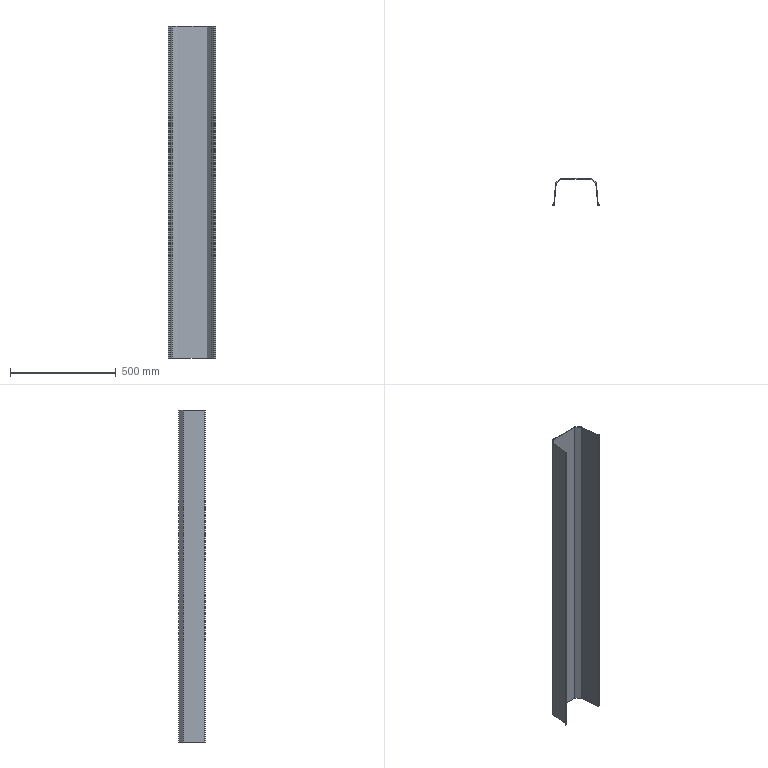Part | STEP file | 51E-01221JG10 | 1 solid | 56 faces | box 225 x 127 x 1570 mm | volume 1681663 mm3 | plane 40 | cylinder 16 | commonest cylinder face diameters 2 x6 7 x6 2.5 x4
STEP:
#1=CARTESIAN_POINT('',(-106.207,0.,1570.));
#2=VERTEX_POINT('',#1);
#3=CARTESIAN_POINT('',(-106.207,2.5,1570.));
#4=VERTEX_POINT('',#3);
#5=CARTESIAN_POINT('',(-106.207,1.25,1570.));
#6=DIRECTION('',(0.,1.,0.));
#7=VECTOR('',#6,1.);
#8=LINE('',#5,#7);
#9=EDGE_CURVE('',#2,#4,#8,.T.);
#10=ORIENTED_EDGE('',*,*,#9,.F.);
#11=CARTESIAN_POINT('',(-102.72,3.195,1570.));
#12=VERTEX_POINT('',#11);
#13=CARTESIAN_POINT('',(-102.72,3.195,1570.));
#14=CARTESIAN_POINT('',(-102.752,2.83,1570.));
#15=CARTESIAN_POINT('',(-102.832,2.469,1570.));
#16=CARTESIAN_POINT('',(-102.959,2.12,1570.));
#17=CARTESIAN_POINT('',(-103.301,1.465,1570.));
#18=CARTESIAN_POINT('',(-103.8,0.9191,1570.));
#19=CARTESIAN_POINT('',(-104.084,0.6808,1570.));
#20=CARTESIAN_POINT('',(-104.656,0.3172,1570.));
#21=CARTESIAN_POINT('',(-105.296,0.09984,1570.));
#22=CARTESIAN_POINT('',(-105.597,0.03328,1570.));
#23=CARTESIAN_POINT('',(-105.902,0.,1570.));
#24=CARTESIAN_POINT('',(-106.207,0.,1570.));
#25=B_SPLINE_CURVE_WITH_KNOTS('',5,(#13,#14,#15,#16,#17,#18,#19,#20,#21,#22,#23,#24),.UNSPECIFIED.,.F.,.U.,(6,3,3,6),(0.,2.592,5.185,7.343),.UNSPECIFIED.);
#26=EDGE_CURVE('',#12,#2,#25,.T.);
#27=ORIENTED_EDGE('',*,*,#26,.F.);
#28=CARTESIAN_POINT('',(-105.211,3.413,1570.));
#29=VERTEX_POINT('',#28);
#30=CARTESIAN_POINT('',(-103.966,3.304,1570.));
#31=DIRECTION('',(0.9962,-0.08716,0.));
#32=VECTOR('',#31,1.);
#33=LINE('',#30,#32);
#34=EDGE_CURVE('',#29,#12,#33,.T.);
#35=ORIENTED_EDGE('',*,*,#34,.F.);
#36=CARTESIAN_POINT('',(-105.211,3.413,1570.));
#37=CARTESIAN_POINT('',(-105.22,3.315,1570.));
#38=CARTESIAN_POINT('',(-105.24,3.219,1570.));
#39=CARTESIAN_POINT('',(-105.272,3.125,1570.));
#40=CARTESIAN_POINT('',(-105.359,2.948,1570.));
#41=CARTESIAN_POINT('',(-105.486,2.797,1570.));
#42=CARTESIAN_POINT('',(-105.559,2.729,1570.));
#43=CARTESIAN_POINT('',(-105.719,2.614,1570.));
#44=CARTESIAN_POINT('',(-105.902,2.54,1570.));
#45=CARTESIAN_POINT('',(-105.998,2.515,1570.));
#46=CARTESIAN_POINT('',(-106.098,2.501,1570.));
#47=CARTESIAN_POINT('',(-106.199,2.5,1570.));
#48=CARTESIAN_POINT('',(-106.202,2.5,1570.));
#49=CARTESIAN_POINT('',(-106.204,2.5,1570.));
#50=CARTESIAN_POINT('',(-106.207,2.5,1570.));
#51=B_SPLINE_CURVE_WITH_KNOTS('',5,(#36,#37,#38,#39,#40,#41,#42,#43,#44,#45,#46,#47,#48,#49,#50),.UNSPECIFIED.,.F.,.U.,(6,3,3,3,6),(0.,0.6928,1.386,2.078,2.098),.UNSPECIFIED.);
#52=EDGE_CURVE('',#29,#4,#51,.T.);
#53=ORIENTED_EDGE('',*,*,#52,.T.);
#54=EDGE_LOOP('',(#10,#27,#35,#53));
#55=FACE_OUTER_BOUND('',#54,.T.);
#56=CARTESIAN_POINT('',(-106.207,0.,1570.));
#57=DIRECTION('',(0.,0.,1.));
#58=DIRECTION('',(1.,0.,0.));
#59=AXIS2_PLACEMENT_3D('',#56,#57,#58);
#60=PLANE('',#59);
#61=ADVANCED_FACE('',(#55),#60,.T.);
#62=CARTESIAN_POINT('',(-111.25,2.5,1570.));
#63=VERTEX_POINT('',#62);
#64=CARTESIAN_POINT('',(-112.5,1.25,1570.));
#65=VERTEX_POINT('',#64);
#66=CARTESIAN_POINT('',(-111.25,1.25,1570.));
#67=DIRECTION('',(0.,0.,1.));
#68=AXIS2_PLACEMENT_3D('',#66,#67,$);
#69=CIRCLE('',#68,1.25);
#70=EDGE_CURVE('',#63,#65,#69,.T.);
#71=ORIENTED_EDGE('',*,*,#70,.T.);
#72=CARTESIAN_POINT('',(-111.25,0.,1570.));
#73=VERTEX_POINT('',#72);
#74=CARTESIAN_POINT('',(-111.25,1.25,1570.));
#75=DIRECTION('',(0.,0.,1.));
#76=AXIS2_PLACEMENT_3D('',#74,#75,$);
#77=CIRCLE('',#76,1.25);
#78=EDGE_CURVE('',#65,#73,#77,.T.);
#79=ORIENTED_EDGE('',*,*,#78,.T.);
#80=CARTESIAN_POINT('',(-108.729,0.,1570.));
#81=DIRECTION('',(-1.,0.,0.));
#82=VECTOR('',#81,1.);
#83=LINE('',#80,#82);
#84=EDGE_CURVE('',#2,#73,#83,.T.);
#85=ORIENTED_EDGE('',*,*,#84,.F.);
#86=ORIENTED_EDGE('',*,*,#9,.T.);
#87=CARTESIAN_POINT('',(-108.729,2.5,1570.));
#88=DIRECTION('',(-1.,0.,0.));
#89=VECTOR('',#88,1.);
#90=LINE('',#87,#89);
#91=EDGE_CURVE('',#4,#63,#90,.T.);
#92=ORIENTED_EDGE('',*,*,#91,.T.);
#93=EDGE_LOOP('',(#71,#79,#85,#86,#92));
#94=FACE_OUTER_BOUND('',#93,.T.);
#95=CARTESIAN_POINT('',(-105.211,3.413,1570.));
#96=DIRECTION('',(0.,0.,1.));
#97=DIRECTION('',(1.,0.,0.));
#98=AXIS2_PLACEMENT_3D('',#95,#96,#97);
#99=PLANE('',#98);
#100=ADVANCED_FACE('',(#94),#99,.T.);
#101=CARTESIAN_POINT('',(-102.72,3.195,0.));
#102=VERTEX_POINT('',#101);
#103=CARTESIAN_POINT('',(-106.207,0.,0.));
#104=VERTEX_POINT('',#103);
#105=CARTESIAN_POINT('',(-106.207,3.5,0.));
#106=DIRECTION('',(0.,0.,-1.));
#107=AXIS2_PLACEMENT_3D('',#105,#106,$);
#108=CIRCLE('',#107,3.5);
#109=EDGE_CURVE('',#102,#104,#108,.T.);
#110=ORIENTED_EDGE('',*,*,#109,.F.);
#111=CARTESIAN_POINT('',(-102.72,3.195,1570.));
#112=DIRECTION('',(0.,0.,-1.));
#113=VECTOR('',#112,1.);
#114=LINE('',#111,#113);
#115=EDGE_CURVE('',#12,#102,#114,.T.);
#116=ORIENTED_EDGE('',*,*,#115,.F.);
#117=ORIENTED_EDGE('',*,*,#26,.T.);
#118=CARTESIAN_POINT('',(-106.207,0.,1570.));
#119=DIRECTION('',(0.,0.,-1.));
#120=VECTOR('',#119,1.);
#121=LINE('',#118,#120);
#122=EDGE_CURVE('',#2,#104,#121,.T.);
#123=ORIENTED_EDGE('',*,*,#122,.T.);
#124=EDGE_LOOP('',(#110,#116,#117,#123));
#125=FACE_OUTER_BOUND('',#124,.T.);
#126=CARTESIAN_POINT('',(-106.207,3.5,1570.));
#127=DIRECTION('',(0.,0.,-1.));
#128=DIRECTION('',(1.,0.,0.));
#129=AXIS2_PLACEMENT_3D('',#126,#127,#128);
#130=CYLINDRICAL_SURFACE('',#129,3.5);
#131=ADVANCED_FACE('',(#125),#130,.T.);
#132=CARTESIAN_POINT('',(-94.02,102.637,1570.));
#133=VERTEX_POINT('',#132);
#134=CARTESIAN_POINT('',(-98.37,52.916,1570.));
#135=DIRECTION('',(-0.08716,-0.9962,0.));
#136=VECTOR('',#135,1.);
#137=LINE('',#134,#136);
#138=EDGE_CURVE('',#133,#12,#137,.T.);
#139=ORIENTED_EDGE('',*,*,#138,.F.);
#140=CARTESIAN_POINT('',(-96.511,102.855,1570.));
#141=VERTEX_POINT('',#140);
#142=CARTESIAN_POINT('',(-95.266,102.746,1570.));
#143=DIRECTION('',(-0.9962,0.08716,0.));
#144=VECTOR('',#143,1.);
#145=LINE('',#142,#144);
#146=EDGE_CURVE('',#133,#141,#145,.T.);
#147=ORIENTED_EDGE('',*,*,#146,.T.);
#148=CARTESIAN_POINT('',(-100.861,53.134,1570.));
#149=DIRECTION('',(-0.08716,-0.9962,0.));
#150=VECTOR('',#149,1.);
#151=LINE('',#148,#150);
#152=EDGE_CURVE('',#141,#29,#151,.T.);
#153=ORIENTED_EDGE('',*,*,#152,.T.);
#154=ORIENTED_EDGE('',*,*,#34,.T.);
#155=EDGE_LOOP('',(#139,#147,#153,#154));
#156=FACE_OUTER_BOUND('',#155,.T.);
#157=CARTESIAN_POINT('',(-95.499,105.025,1570.));
#158=DIRECTION('',(0.,0.,1.));
#159=DIRECTION('',(1.,0.,0.));
#160=AXIS2_PLACEMENT_3D('',#157,#158,#159);
#161=PLANE('',#160);
#162=ADVANCED_FACE('',(#156),#161,.T.);
#163=CARTESIAN_POINT('',(-105.211,3.413,0.));
#164=VERTEX_POINT('',#163);
#165=CARTESIAN_POINT('',(-106.207,2.5,0.));
#166=VERTEX_POINT('',#165);
#167=CARTESIAN_POINT('',(-106.207,3.5,0.));
#168=DIRECTION('',(0.,0.,-1.));
#169=AXIS2_PLACEMENT_3D('',#167,#168,$);
#170=CIRCLE('',#169,1.);
#171=EDGE_CURVE('',#164,#166,#170,.T.);
#172=ORIENTED_EDGE('',*,*,#171,.T.);
#173=CARTESIAN_POINT('',(-106.207,2.5,1570.));
#174=DIRECTION('',(0.,0.,-1.));
#175=VECTOR('',#174,1.);
#176=LINE('',#173,#175);
#177=EDGE_CURVE('',#4,#166,#176,.T.);
#178=ORIENTED_EDGE('',*,*,#177,.F.);
#179=ORIENTED_EDGE('',*,*,#52,.F.);
#180=CARTESIAN_POINT('',(-105.211,3.413,1570.));
#181=DIRECTION('',(0.,0.,-1.));
#182=VECTOR('',#181,1.);
#183=LINE('',#180,#182);
#184=EDGE_CURVE('',#29,#164,#183,.T.);
#185=ORIENTED_EDGE('',*,*,#184,.T.);
#186=EDGE_LOOP('',(#172,#178,#179,#185));
#187=FACE_OUTER_BOUND('',#186,.T.);
#188=CARTESIAN_POINT('',(-106.207,3.5,1570.));
#189=DIRECTION('',(0.,0.,-1.));
#190=DIRECTION('',(1.,0.,0.));
#191=AXIS2_PLACEMENT_3D('',#188,#189,#190);
#192=CYLINDRICAL_SURFACE('',#191,1.);
#193=ADVANCED_FACE('',(#187),#192,.F.);
#194=CARTESIAN_POINT('',(-112.5,1.25,0.));
#195=VERTEX_POINT('',#194);
#196=CARTESIAN_POINT('',(-112.5,1.25,1570.));
#197=DIRECTION('',(0.,0.,1.));
#198=VECTOR('',#197,1.);
#199=LINE('',#196,#198);
#200=EDGE_CURVE('',#65,#195,#199,.F.);
#201=ORIENTED_EDGE('',*,*,#200,.F.);
#202=ORIENTED_EDGE('',*,*,#70,.F.);
#203=CARTESIAN_POINT('',(-111.25,2.5,0.));
#204=VERTEX_POINT('',#203);
#205=CARTESIAN_POINT('',(-111.25,2.5,1570.));
#206=DIRECTION('',(0.,0.,1.));
#207=VECTOR('',#206,1.);
#208=LINE('',#205,#207);
#209=EDGE_CURVE('',#204,#63,#208,.T.);
#210=ORIENTED_EDGE('',*,*,#209,.F.);
#211=CARTESIAN_POINT('',(-111.25,1.25,0.));
#212=DIRECTION('',(0.,0.,1.));
#213=AXIS2_PLACEMENT_3D('',#211,#212,$);
#214=CIRCLE('',#213,1.25);
#215=EDGE_CURVE('',#195,#204,#214,.F.);
#216=ORIENTED_EDGE('',*,*,#215,.F.);
#217=EDGE_LOOP('',(#201,#202,#210,#216));
#218=FACE_OUTER_BOUND('',#217,.T.);
#219=CARTESIAN_POINT('',(-111.25,1.25,1570.));
#220=DIRECTION('',(0.,0.,1.));
#221=DIRECTION('',(1.,0.,0.));
#222=AXIS2_PLACEMENT_3D('',#219,#220,#221);
#223=CYLINDRICAL_SURFACE('',#222,1.25);
#224=ADVANCED_FACE('',(#218),#223,.T.);
#225=ORIENTED_EDGE('',*,*,#78,.F.);
#226=ORIENTED_EDGE('',*,*,#200,.T.);
#227=CARTESIAN_POINT('',(-111.25,0.,0.));
#228=VERTEX_POINT('',#227);
#229=CARTESIAN_POINT('',(-111.25,1.25,0.));
#230=DIRECTION('',(0.,0.,-1.));
#231=AXIS2_PLACEMENT_3D('',#229,#230,$);
#232=CIRCLE('',#231,1.25);
#233=EDGE_CURVE('',#228,#195,#232,.T.);
#234=ORIENTED_EDGE('',*,*,#233,.F.);
#235=CARTESIAN_POINT('',(-111.25,0.,1570.));
#236=DIRECTION('',(0.,0.,-1.));
#237=VECTOR('',#236,1.);
#238=LINE('',#235,#237);
#239=EDGE_CURVE('',#73,#228,#238,.T.);
#240=ORIENTED_EDGE('',*,*,#239,.F.);
#241=EDGE_LOOP('',(#225,#226,#234,#240));
#242=FACE_OUTER_BOUND('',#241,.T.);
#243=CARTESIAN_POINT('',(-111.25,1.25,1570.));
#244=DIRECTION('',(0.,0.,-1.));
#245=DIRECTION('',(1.,0.,0.));
#246=AXIS2_PLACEMENT_3D('',#243,#244,#245);
#247=CYLINDRICAL_SURFACE('',#246,1.25);
#248=ADVANCED_FACE('',(#242),#247,.T.);
#249=ORIENTED_EDGE('',*,*,#84,.T.);
#250=ORIENTED_EDGE('',*,*,#239,.T.);
#251=CARTESIAN_POINT('',(-108.729,0.,0.));
#252=DIRECTION('',(-1.,0.,0.));
#253=VECTOR('',#252,1.);
#254=LINE('',#251,#253);
#255=EDGE_CURVE('',#104,#228,#254,.T.);
#256=ORIENTED_EDGE('',*,*,#255,.F.);
#257=ORIENTED_EDGE('',*,*,#122,.F.);
#258=EDGE_LOOP('',(#249,#250,#256,#257));
#259=FACE_OUTER_BOUND('',#258,.T.);
#260=CARTESIAN_POINT('',(-112.5,0.,1570.));
#261=DIRECTION('',(0.,-1.,0.));
#262=DIRECTION('',(0.,0.,-1.));
#263=AXIS2_PLACEMENT_3D('',#260,#261,#262);
#264=PLANE('',#263);
#265=ADVANCED_FACE('',(#259),#264,.T.);
#266=CARTESIAN_POINT('',(-108.729,2.5,0.));
#267=DIRECTION('',(-1.,0.,0.));
#268=VECTOR('',#267,1.);
#269=LINE('',#266,#268);
#270=EDGE_CURVE('',#166,#204,#269,.T.);
#271=ORIENTED_EDGE('',*,*,#270,.T.);
#272=ORIENTED_EDGE('',*,*,#209,.T.);
#273=ORIENTED_EDGE('',*,*,#91,.F.);
#274=ORIENTED_EDGE('',*,*,#177,.T.);
#275=EDGE_LOOP('',(#271,#272,#273,#274));
#276=FACE_OUTER_BOUND('',#275,.T.);
#277=CARTESIAN_POINT('',(-112.5,2.5,1570.));
#278=DIRECTION('',(0.,-1.,0.));
#279=DIRECTION('',(0.,0.,-1.));
#280=AXIS2_PLACEMENT_3D('',#277,#278,#279);
#281=PLANE('',#280);
#282=ADVANCED_FACE('',(#276),#281,.F.);
#283=CARTESIAN_POINT('',(-103.966,3.304,0.));
#284=DIRECTION('',(-0.9962,0.08716,0.));
#285=VECTOR('',#284,1.);
#286=LINE('',#283,#285);
#287=EDGE_CURVE('',#102,#164,#286,.T.);
#288=ORIENTED_EDGE('',*,*,#287,.F.);
#289=ORIENTED_EDGE('',*,*,#109,.T.);
#290=CARTESIAN_POINT('',(-106.207,1.25,0.));
#291=DIRECTION('',(0.,-1.,0.));
#292=VECTOR('',#291,1.);
#293=LINE('',#290,#292);
#294=EDGE_CURVE('',#166,#104,#293,.T.);
#295=ORIENTED_EDGE('',*,*,#294,.F.);
#296=ORIENTED_EDGE('',*,*,#171,.F.);
#297=EDGE_LOOP('',(#288,#289,#295,#296));
#298=FACE_OUTER_BOUND('',#297,.T.);
#299=CARTESIAN_POINT('',(-102.72,3.195,0.));
#300=DIRECTION('',(0.,0.,-1.));
#301=DIRECTION('',(-1.,0.,0.));
#302=AXIS2_PLACEMENT_3D('',#299,#300,#301);
#303=PLANE('',#302);
#304=ADVANCED_FACE('',(#298),#303,.T.);
#305=CARTESIAN_POINT('',(-94.02,102.637,0.));
#306=VERTEX_POINT('',#305);
#307=CARTESIAN_POINT('',(-98.37,52.916,0.));
#308=DIRECTION('',(-0.08716,-0.9962,0.));
#309=VECTOR('',#308,1.);
#310=LINE('',#307,#309);
#311=EDGE_CURVE('',#306,#102,#310,.T.);
#312=ORIENTED_EDGE('',*,*,#311,.F.);
#313=CARTESIAN_POINT('',(-94.02,102.637,785.));
#314=DIRECTION('',(0.,0.,-1.));
#315=VECTOR('',#314,1.);
#316=LINE('',#313,#315);
#317=EDGE_CURVE('',#133,#306,#316,.T.);
#318=ORIENTED_EDGE('',*,*,#317,.F.);
#319=ORIENTED_EDGE('',*,*,#138,.T.);
#320=ORIENTED_EDGE('',*,*,#115,.T.);
#321=EDGE_LOOP('',(#312,#318,#319,#320));
#322=FACE_OUTER_BOUND('',#321,.T.);
#323=CARTESIAN_POINT('',(-103.,0.,1570.));
#324=DIRECTION('',(0.9962,-0.08716,0.));
#325=DIRECTION('',(0.08716,0.9962,0.));
#326=AXIS2_PLACEMENT_3D('',#323,#324,#325);
#327=PLANE('',#326);
#328=ADVANCED_FACE('',(#322),#327,.T.);
#329=ORIENTED_EDGE('',*,*,#146,.F.);
#330=CARTESIAN_POINT('',(-93.731,103.257,1570.));
#331=VERTEX_POINT('',#330);
#332=CARTESIAN_POINT('',(-93.024,102.55,1570.));
#333=DIRECTION('',(0.,0.,1.));
#334=AXIS2_PLACEMENT_3D('',#332,#333,$);
#335=CIRCLE('',#334,1.);
#336=EDGE_CURVE('',#331,#133,#335,.T.);
#337=ORIENTED_EDGE('',*,*,#336,.F.);
#338=CARTESIAN_POINT('',(-95.499,105.025,1570.));
#339=VERTEX_POINT('',#338);
#340=CARTESIAN_POINT('',(-94.615,104.141,1570.));
#341=DIRECTION('',(0.7071,-0.7071,0.));
#342=VECTOR('',#341,1.);
#343=LINE('',#340,#342);
#344=EDGE_CURVE('',#339,#331,#343,.T.);
#345=ORIENTED_EDGE('',*,*,#344,.F.);
#346=CARTESIAN_POINT('',(-93.024,102.55,1570.));
#347=DIRECTION('',(0.,0.,1.));
#348=AXIS2_PLACEMENT_3D('',#346,#347,$);
#349=CIRCLE('',#348,3.5);
#350=EDGE_CURVE('',#339,#141,#349,.T.);
#351=ORIENTED_EDGE('',*,*,#350,.T.);
#352=EDGE_LOOP('',(#329,#337,#345,#351));
#353=FACE_OUTER_BOUND('',#352,.T.);
#354=CARTESIAN_POINT('',(-94.02,102.637,1570.));
#355=DIRECTION('',(0.,0.,1.));
#356=DIRECTION('',(1.,0.,0.));
#357=AXIS2_PLACEMENT_3D('',#354,#355,#356);
#358=PLANE('',#357);
#359=ADVANCED_FACE('',(#353),#358,.T.);
#360=CARTESIAN_POINT('',(-96.511,102.855,0.));
#361=VERTEX_POINT('',#360);
#362=CARTESIAN_POINT('',(-100.861,53.134,0.));
#363=DIRECTION('',(-0.08716,-0.9962,0.));
#364=VECTOR('',#363,1.);
#365=LINE('',#362,#364);
#366=EDGE_CURVE('',#361,#164,#365,.T.);
#367=ORIENTED_EDGE('',*,*,#366,.T.);
#368=ORIENTED_EDGE('',*,*,#184,.F.);
#369=ORIENTED_EDGE('',*,*,#152,.F.);
#370=CARTESIAN_POINT('',(-96.511,102.855,785.));
#371=DIRECTION('',(0.,0.,-1.));
#372=VECTOR('',#371,1.);
#373=LINE('',#370,#372);
#374=EDGE_CURVE('',#141,#361,#373,.T.);
#375=ORIENTED_EDGE('',*,*,#374,.T.);
#376=EDGE_LOOP('',(#367,#368,#369,#375));
#377=FACE_OUTER_BOUND('',#376,.T.);
#378=CARTESIAN_POINT('',(-105.49,0.2179,1570.));
#379=DIRECTION('',(0.9962,-0.08716,0.));
#380=DIRECTION('',(0.08716,0.9962,0.));
#381=AXIS2_PLACEMENT_3D('',#378,#379,#380);
#382=PLANE('',#381);
#383=ADVANCED_FACE('',(#377),#382,.F.);
#384=ORIENTED_EDGE('',*,*,#255,.T.);
#385=ORIENTED_EDGE('',*,*,#233,.T.);
#386=ORIENTED_EDGE('',*,*,#215,.T.);
#387=ORIENTED_EDGE('',*,*,#270,.F.);
#388=ORIENTED_EDGE('',*,*,#294,.T.);
#389=EDGE_LOOP('',(#384,#385,#386,#387,#388));
#390=FACE_OUTER_BOUND('',#389,.T.);
#391=CARTESIAN_POINT('',(-106.207,3.5,0.));
#392=DIRECTION('',(0.,0.,-1.));
#393=DIRECTION('',(-1.,0.,0.));
#394=AXIS2_PLACEMENT_3D('',#391,#392,#393);
#395=PLANE('',#394);
#396=ADVANCED_FACE('',(#390),#395,.T.);
#397=ORIENTED_EDGE('',*,*,#311,.T.);
#398=ORIENTED_EDGE('',*,*,#287,.T.);
#399=ORIENTED_EDGE('',*,*,#366,.F.);
#400=CARTESIAN_POINT('',(-95.266,102.746,0.));
#401=DIRECTION('',(0.9962,-0.08716,0.));
#402=VECTOR('',#401,1.);
#403=LINE('',#400,#402);
#404=EDGE_CURVE('',#361,#306,#403,.T.);
#405=ORIENTED_EDGE('',*,*,#404,.T.);
#406=EDGE_LOOP('',(#397,#398,#399,#405));
#407=FACE_OUTER_BOUND('',#406,.T.);
#408=CARTESIAN_POINT('',(-106.207,2.5,0.));
#409=DIRECTION('',(0.,0.,-1.));
#410=DIRECTION('',(-1.,0.,0.));
#411=AXIS2_PLACEMENT_3D('',#408,#409,#410);
#412=PLANE('',#411);
#413=ADVANCED_FACE('',(#407),#412,.T.);
#414=CARTESIAN_POINT('',(-93.731,103.257,0.));
#415=VERTEX_POINT('',#414);
#416=CARTESIAN_POINT('',(-93.024,102.55,0.));
#417=DIRECTION('',(0.,0.,-1.));
#418=AXIS2_PLACEMENT_3D('',#416,#417,$);
#419=CIRCLE('',#418,1.);
#420=EDGE_CURVE('',#415,#306,#419,.F.);
#421=ORIENTED_EDGE('',*,*,#420,.F.);
#422=CARTESIAN_POINT('',(-93.731,103.257,1570.));
#423=DIRECTION('',(0.,0.,-1.));
#424=VECTOR('',#423,1.);
#425=LINE('',#422,#424);
#426=EDGE_CURVE('',#331,#415,#425,.T.);
#427=ORIENTED_EDGE('',*,*,#426,.F.);
#428=ORIENTED_EDGE('',*,*,#336,.T.);
#429=ORIENTED_EDGE('',*,*,#317,.T.);
#430=EDGE_LOOP('',(#421,#427,#428,#429));
#431=FACE_OUTER_BOUND('',#430,.T.);
#432=CARTESIAN_POINT('',(-93.024,102.55,1570.));
#433=DIRECTION('',(0.,0.,-1.));
#434=DIRECTION('',(-1.,0.,0.));
#435=AXIS2_PLACEMENT_3D('',#432,#433,#434);
#436=CYLINDRICAL_SURFACE('',#435,1.);
#437=ADVANCED_FACE('',(#431),#436,.F.);
#438=CARTESIAN_POINT('',(-72.782,124.207,1570.));
#439=VERTEX_POINT('',#438);
#440=CARTESIAN_POINT('',(-83.256,113.732,1570.));
#441=DIRECTION('',(-0.7071,-0.7071,0.));
#442=VECTOR('',#441,1.);
#443=LINE('',#440,#442);
#444=EDGE_CURVE('',#439,#331,#443,.T.);
#445=ORIENTED_EDGE('',*,*,#444,.F.);
#446=CARTESIAN_POINT('',(-74.549,125.975,1570.));
#447=VERTEX_POINT('',#446);
#448=CARTESIAN_POINT('',(-73.665,125.091,1570.));
#449=DIRECTION('',(-0.7071,0.7071,0.));
#450=VECTOR('',#449,1.);
#451=LINE('',#448,#450);
#452=EDGE_CURVE('',#439,#447,#451,.T.);
#453=ORIENTED_EDGE('',*,*,#452,.T.);
#454=CARTESIAN_POINT('',(-85.024,115.5,1570.));
#455=DIRECTION('',(-0.7071,-0.7071,0.));
#456=VECTOR('',#455,1.);
#457=LINE('',#454,#456);
#458=EDGE_CURVE('',#447,#339,#457,.T.);
#459=ORIENTED_EDGE('',*,*,#458,.T.);
#460=ORIENTED_EDGE('',*,*,#344,.T.);
#461=EDGE_LOOP('',(#445,#453,#459,#460));
#462=FACE_OUTER_BOUND('',#461,.T.);
#463=CARTESIAN_POINT('',(-72.074,127.,1570.));
#464=DIRECTION('',(0.,0.,1.));
#465=DIRECTION('',(1.,0.,0.));
#466=AXIS2_PLACEMENT_3D('',#463,#464,#465);
#467=PLANE('',#466);
#468=ADVANCED_FACE('',(#462),#467,.T.);
#469=CARTESIAN_POINT('',(-95.499,105.025,0.));
#470=VERTEX_POINT('',#469);
#471=CARTESIAN_POINT('',(-93.024,102.55,0.));
#472=DIRECTION('',(0.,0.,-1.));
#473=AXIS2_PLACEMENT_3D('',#471,#472,$);
#474=CIRCLE('',#473,3.5);
#475=EDGE_CURVE('',#470,#361,#474,.F.);
#476=ORIENTED_EDGE('',*,*,#475,.T.);
#477=ORIENTED_EDGE('',*,*,#374,.F.);
#478=ORIENTED_EDGE('',*,*,#350,.F.);
#479=CARTESIAN_POINT('',(-95.499,105.025,1570.));
#480=DIRECTION('',(0.,0.,-1.));
#481=VECTOR('',#480,1.);
#482=LINE('',#479,#481);
#483=EDGE_CURVE('',#339,#470,#482,.T.);
#484=ORIENTED_EDGE('',*,*,#483,.T.);
#485=EDGE_LOOP('',(#476,#477,#478,#484));
#486=FACE_OUTER_BOUND('',#485,.T.);
#487=CARTESIAN_POINT('',(-93.024,102.55,1570.));
#488=DIRECTION('',(0.,0.,-1.));
#489=DIRECTION('',(-1.,0.,0.));
#490=AXIS2_PLACEMENT_3D('',#487,#488,#489);
#491=CYLINDRICAL_SURFACE('',#490,3.5);
#492=ADVANCED_FACE('',(#486),#491,.T.);
#493=CARTESIAN_POINT('',(-94.615,104.141,0.));
#494=DIRECTION('',(-0.7071,0.7071,0.));
#495=VECTOR('',#494,1.);
#496=LINE('',#493,#495);
#497=EDGE_CURVE('',#415,#470,#496,.T.);
#498=ORIENTED_EDGE('',*,*,#497,.F.);
#499=ORIENTED_EDGE('',*,*,#420,.T.);
#500=ORIENTED_EDGE('',*,*,#404,.F.);
#501=ORIENTED_EDGE('',*,*,#475,.F.);
#502=EDGE_LOOP('',(#498,#499,#500,#501));
#503=FACE_OUTER_BOUND('',#502,.T.);
#504=CARTESIAN_POINT('',(-93.731,103.257,0.));
#505=DIRECTION('',(0.,0.,-1.));
#506=DIRECTION('',(-1.,0.,0.));
#507=AXIS2_PLACEMENT_3D('',#504,#505,#506);
#508=PLANE('',#507);
#509=ADVANCED_FACE('',(#503),#508,.T.);
#510=CARTESIAN_POINT('',(-72.782,124.207,0.));
#511=VERTEX_POINT('',#510);
#512=CARTESIAN_POINT('',(-83.256,113.732,0.));
#513=DIRECTION('',(-0.7071,-0.7071,0.));
#514=VECTOR('',#513,1.);
#515=LINE('',#512,#514);
#516=EDGE_CURVE('',#511,#415,#515,.T.);
#517=ORIENTED_EDGE('',*,*,#516,.F.);
#518=CARTESIAN_POINT('',(-72.782,124.207,785.));
#519=DIRECTION('',(0.,0.,-1.));
#520=VECTOR('',#519,1.);
#521=LINE('',#518,#520);
#522=EDGE_CURVE('',#439,#511,#521,.T.);
#523=ORIENTED_EDGE('',*,*,#522,.F.);
#524=ORIENTED_EDGE('',*,*,#444,.T.);
#525=ORIENTED_EDGE('',*,*,#426,.T.);
#526=EDGE_LOOP('',(#517,#523,#524,#525));
#527=FACE_OUTER_BOUND('',#526,.T.);
#528=CARTESIAN_POINT('',(-93.989,103.,1570.));
#529=DIRECTION('',(0.7071,-0.7071,0.));
#530=DIRECTION('',(0.7071,0.7071,0.));
#531=AXIS2_PLACEMENT_3D('',#528,#529,#530);
#532=PLANE('',#531);
#533=ADVANCED_FACE('',(#527),#532,.T.);
#534=ORIENTED_EDGE('',*,*,#452,.F.);
#535=CARTESIAN_POINT('',(-72.074,124.5,1570.));
#536=VERTEX_POINT('',#535);
#537=CARTESIAN_POINT('',(-72.074,123.5,1570.));
#538=DIRECTION('',(0.,0.,1.));
#539=AXIS2_PLACEMENT_3D('',#537,#538,$);
#540=CIRCLE('',#539,1.);
#541=EDGE_CURVE('',#536,#439,#540,.T.);
#542=ORIENTED_EDGE('',*,*,#541,.F.);
#543=CARTESIAN_POINT('',(-72.074,127.,1570.));
#544=VERTEX_POINT('',#543);
#545=CARTESIAN_POINT('',(-72.074,125.75,1570.));
#546=DIRECTION('',(0.,-1.,0.));
#547=VECTOR('',#546,1.);
#548=LINE('',#545,#547);
#549=EDGE_CURVE('',#544,#536,#548,.T.);
#550=ORIENTED_EDGE('',*,*,#549,.F.);
#551=CARTESIAN_POINT('',(-72.074,123.5,1570.));
#552=DIRECTION('',(0.,0.,1.));
#553=AXIS2_PLACEMENT_3D('',#551,#552,$);
#554=CIRCLE('',#553,3.5);
#555=EDGE_CURVE('',#544,#447,#554,.T.);
#556=ORIENTED_EDGE('',*,*,#555,.T.);
#557=EDGE_LOOP('',(#534,#542,#550,#556));
#558=FACE_OUTER_BOUND('',#557,.T.);
#559=CARTESIAN_POINT('',(-72.782,124.207,1570.));
#560=DIRECTION('',(0.,0.,1.));
#561=DIRECTION('',(1.,0.,0.));
#562=AXIS2_PLACEMENT_3D('',#559,#560,#561);
#563=PLANE('',#562);
#564=ADVANCED_FACE('',(#558),#563,.T.);
#565=CARTESIAN_POINT('',(-74.549,125.975,0.));
#566=VERTEX_POINT('',#565);
#567=CARTESIAN_POINT('',(-85.024,115.5,0.));
#568=DIRECTION('',(-0.7071,-0.7071,0.));
#569=VECTOR('',#568,1.);
#570=LINE('',#567,#569);
#571=EDGE_CURVE('',#566,#470,#570,.T.);
#572=ORIENTED_EDGE('',*,*,#571,.T.);
#573=ORIENTED_EDGE('',*,*,#483,.F.);
#574=ORIENTED_EDGE('',*,*,#458,.F.);
#575=CARTESIAN_POINT('',(-74.549,125.975,785.));
#576=DIRECTION('',(0.,0.,-1.));
#577=VECTOR('',#576,1.);
#578=LINE('',#575,#577);
#579=EDGE_CURVE('',#447,#566,#578,.T.);
#580=ORIENTED_EDGE('',*,*,#579,.T.);
#581=EDGE_LOOP('',(#572,#573,#574,#580));
#582=FACE_OUTER_BOUND('',#581,.T.);
#583=CARTESIAN_POINT('',(-95.756,104.768,1570.));
#584=DIRECTION('',(0.7071,-0.7071,0.));
#585=DIRECTION('',(0.7071,0.7071,0.));
#586=AXIS2_PLACEMENT_3D('',#583,#584,#585);
#587=PLANE('',#586);
#588=ADVANCED_FACE('',(#582),#587,.F.);
#589=ORIENTED_EDGE('',*,*,#516,.T.);
#590=ORIENTED_EDGE('',*,*,#497,.T.);
#591=ORIENTED_EDGE('',*,*,#571,.F.);
#592=CARTESIAN_POINT('',(-73.665,125.091,0.));
#593=DIRECTION('',(0.7071,-0.7071,0.));
#594=VECTOR('',#593,1.);
#595=LINE('',#592,#594);
#596=EDGE_CURVE('',#566,#511,#595,.T.);
#597=ORIENTED_EDGE('',*,*,#596,.T.);
#598=EDGE_LOOP('',(#589,#590,#591,#597));
#599=FACE_OUTER_BOUND('',#598,.T.);
#600=CARTESIAN_POINT('',(-96.511,102.855,0.));
#601=DIRECTION('',(0.,0.,-1.));
#602=DIRECTION('',(-1.,0.,0.));
#603=AXIS2_PLACEMENT_3D('',#600,#601,#602);
#604=PLANE('',#603);
#605=ADVANCED_FACE('',(#599),#604,.T.);
#606=CARTESIAN_POINT('',(-72.074,124.5,0.));
#607=VERTEX_POINT('',#606);
#608=CARTESIAN_POINT('',(-72.074,123.5,0.));
#609=DIRECTION('',(0.,0.,-1.));
#610=AXIS2_PLACEMENT_3D('',#608,#609,$);
#611=CIRCLE('',#610,1.);
#612=EDGE_CURVE('',#607,#511,#611,.F.);
#613=ORIENTED_EDGE('',*,*,#612,.F.);
#614=CARTESIAN_POINT('',(-72.074,124.5,1570.));
#615=DIRECTION('',(0.,0.,-1.));
#616=VECTOR('',#615,1.);
#617=LINE('',#614,#616);
#618=EDGE_CURVE('',#536,#607,#617,.T.);
#619=ORIENTED_EDGE('',*,*,#618,.F.);
#620=ORIENTED_EDGE('',*,*,#541,.T.);
#621=ORIENTED_EDGE('',*,*,#522,.T.);
#622=EDGE_LOOP('',(#613,#619,#620,#621));
#623=FACE_OUTER_BOUND('',#622,.T.);
#624=CARTESIAN_POINT('',(-72.074,123.5,1570.));
#625=DIRECTION('',(0.,0.,-1.));
#626=DIRECTION('',(-1.,0.,0.));
#627=AXIS2_PLACEMENT_3D('',#624,#625,#626);
#628=CYLINDRICAL_SURFACE('',#627,1.);
#629=ADVANCED_FACE('',(#623),#628,.F.);
#630=CARTESIAN_POINT('',(72.074,124.5,1570.));
#631=VERTEX_POINT('',#630);
#632=CARTESIAN_POINT('',(0.,124.5,1570.));
#633=DIRECTION('',(-1.,0.,0.));
#634=VECTOR('',#633,1.);
#635=LINE('',#632,#634);
#636=EDGE_CURVE('',#631,#536,#635,.T.);
#637=ORIENTED_EDGE('',*,*,#636,.F.);
#638=CARTESIAN_POINT('',(72.074,127.,1570.));
#639=VERTEX_POINT('',#638);
#640=CARTESIAN_POINT('',(72.074,125.75,1570.));
#641=DIRECTION('',(0.,1.,0.));
#642=VECTOR('',#641,1.);
#643=LINE('',#640,#642);
#644=EDGE_CURVE('',#631,#639,#643,.T.);
#645=ORIENTED_EDGE('',*,*,#644,.T.);
#646=CARTESIAN_POINT('',(0.,127.,1570.));
#647=DIRECTION('',(-1.,0.,0.));
#648=VECTOR('',#647,1.);
#649=LINE('',#646,#648);
#650=EDGE_CURVE('',#639,#544,#649,.T.);
#651=ORIENTED_EDGE('',*,*,#650,.T.);
#652=ORIENTED_EDGE('',*,*,#549,.T.);
#653=EDGE_LOOP('',(#637,#645,#651,#652));
#654=FACE_OUTER_BOUND('',#653,.T.);
#655=CARTESIAN_POINT('',(74.549,125.975,1570.));
#656=DIRECTION('',(0.,0.,1.));
#657=DIRECTION('',(1.,0.,0.));
#658=AXIS2_PLACEMENT_3D('',#655,#656,#657);
#659=PLANE('',#658);
#660=ADVANCED_FACE('',(#654),#659,.T.);
#661=CARTESIAN_POINT('',(-72.074,127.,0.));
#662=VERTEX_POINT('',#661);
#663=CARTESIAN_POINT('',(-72.074,123.5,0.));
#664=DIRECTION('',(0.,0.,-1.));
#665=AXIS2_PLACEMENT_3D('',#663,#664,$);
#666=CIRCLE('',#665,3.5);
#667=EDGE_CURVE('',#662,#566,#666,.F.);
#668=ORIENTED_EDGE('',*,*,#667,.T.);
#669=ORIENTED_EDGE('',*,*,#579,.F.);
#670=ORIENTED_EDGE('',*,*,#555,.F.);
#671=CARTESIAN_POINT('',(-72.074,127.,1570.));
#672=DIRECTION('',(0.,0.,-1.));
#673=VECTOR('',#672,1.);
#674=LINE('',#671,#673);
#675=EDGE_CURVE('',#544,#662,#674,.T.);
#676=ORIENTED_EDGE('',*,*,#675,.T.);
#677=EDGE_LOOP('',(#668,#669,#670,#676));
#678=FACE_OUTER_BOUND('',#677,.T.);
#679=CARTESIAN_POINT('',(-72.074,123.5,1570.));
#680=DIRECTION('',(0.,0.,-1.));
#681=DIRECTION('',(-1.,0.,0.));
#682=AXIS2_PLACEMENT_3D('',#679,#680,#681);
#683=CYLINDRICAL_SURFACE('',#682,3.5);
#684=ADVANCED_FACE('',(#678),#683,.T.);
#685=CARTESIAN_POINT('',(-72.074,125.75,0.));
#686=DIRECTION('',(0.,1.,0.));
#687=VECTOR('',#686,1.);
#688=LINE('',#685,#687);
#689=EDGE_CURVE('',#607,#662,#688,.T.);
#690=ORIENTED_EDGE('',*,*,#689,.F.);
#691=ORIENTED_EDGE('',*,*,#612,.T.);
#692=ORIENTED_EDGE('',*,*,#596,.F.);
#693=ORIENTED_EDGE('',*,*,#667,.F.);
#694=EDGE_LOOP('',(#690,#691,#692,#693));
#695=FACE_OUTER_BOUND('',#694,.T.);
#696=CARTESIAN_POINT('',(-72.074,124.5,0.));
#697=DIRECTION('',(0.,0.,-1.));
#698=DIRECTION('',(-1.,0.,0.));
#699=AXIS2_PLACEMENT_3D('',#696,#697,#698);
#700=PLANE('',#699);
#701=ADVANCED_FACE('',(#695),#700,.T.);
#702=CARTESIAN_POINT('',(72.074,124.5,0.));
#703=VERTEX_POINT('',#702);
#704=CARTESIAN_POINT('',(0.,124.5,0.));
#705=DIRECTION('',(-1.,0.,0.));
#706=VECTOR('',#705,1.);
#707=LINE('',#704,#706);
#708=EDGE_CURVE('',#703,#607,#707,.T.);
#709=ORIENTED_EDGE('',*,*,#708,.F.);
#710=CARTESIAN_POINT('',(72.074,124.5,785.));
#711=DIRECTION('',(0.,0.,-1.));
#712=VECTOR('',#711,1.);
#713=LINE('',#710,#712);
#714=EDGE_CURVE('',#631,#703,#713,.T.);
#715=ORIENTED_EDGE('',*,*,#714,.F.);
#716=ORIENTED_EDGE('',*,*,#636,.T.);
#717=ORIENTED_EDGE('',*,*,#618,.T.);
#718=EDGE_LOOP('',(#709,#715,#716,#717));
#719=FACE_OUTER_BOUND('',#718,.T.);
#720=CARTESIAN_POINT('',(-72.489,124.5,1570.));
#721=DIRECTION('',(0.,-1.,0.));
#722=DIRECTION('',(0.,0.,-1.));
#723=AXIS2_PLACEMENT_3D('',#720,#721,#722);
#724=PLANE('',#723);
#725=ADVANCED_FACE('',(#719),#724,.T.);
#726=ORIENTED_EDGE('',*,*,#644,.F.);
#727=CARTESIAN_POINT('',(72.782,124.207,1570.));
#728=VERTEX_POINT('',#727);
#729=CARTESIAN_POINT('',(72.074,123.5,1570.));
#730=DIRECTION('',(0.,0.,1.));
#731=AXIS2_PLACEMENT_3D('',#729,#730,$);
#732=CIRCLE('',#731,1.);
#733=EDGE_CURVE('',#728,#631,#732,.T.);
#734=ORIENTED_EDGE('',*,*,#733,.F.);
#735=CARTESIAN_POINT('',(74.549,125.975,1570.));
#736=VERTEX_POINT('',#735);
#737=CARTESIAN_POINT('',(73.665,125.091,1570.));
#738=DIRECTION('',(-0.7071,-0.7071,0.));
#739=VECTOR('',#738,1.);
#740=LINE('',#737,#739);
#741=EDGE_CURVE('',#736,#728,#740,.T.);
#742=ORIENTED_EDGE('',*,*,#741,.F.);
#743=CARTESIAN_POINT('',(72.074,123.5,1570.));
#744=DIRECTION('',(0.,0.,1.));
#745=AXIS2_PLACEMENT_3D('',#743,#744,$);
#746=CIRCLE('',#745,3.5);
#747=EDGE_CURVE('',#736,#639,#746,.T.);
#748=ORIENTED_EDGE('',*,*,#747,.T.);
#749=EDGE_LOOP('',(#726,#734,#742,#748));
#750=FACE_OUTER_BOUND('',#749,.T.);
#751=CARTESIAN_POINT('',(72.074,124.5,1570.));
#752=DIRECTION('',(0.,0.,1.));
#753=DIRECTION('',(1.,0.,0.));
#754=AXIS2_PLACEMENT_3D('',#751,#752,#753);
#755=PLANE('',#754);
#756=ADVANCED_FACE('',(#750),#755,.T.);
#757=CARTESIAN_POINT('',(72.074,127.,0.));
#758=VERTEX_POINT('',#757);
#759=CARTESIAN_POINT('',(0.,127.,0.));
#760=DIRECTION('',(-1.,0.,0.));
#761=VECTOR('',#760,1.);
#762=LINE('',#759,#761);
#763=EDGE_CURVE('',#758,#662,#762,.T.);
#764=ORIENTED_EDGE('',*,*,#763,.T.);
#765=ORIENTED_EDGE('',*,*,#675,.F.);
#766=ORIENTED_EDGE('',*,*,#650,.F.);
#767=CARTESIAN_POINT('',(72.074,127.,785.));
#768=DIRECTION('',(0.,0.,-1.));
#769=VECTOR('',#768,1.);
#770=LINE('',#767,#769);
#771=EDGE_CURVE('',#639,#758,#770,.T.);
#772=ORIENTED_EDGE('',*,*,#771,.T.);
#773=EDGE_LOOP('',(#764,#765,#766,#772));
#774=FACE_OUTER_BOUND('',#773,.T.);
#775=CARTESIAN_POINT('',(-72.489,127.,1570.));
#776=DIRECTION('',(0.,-1.,0.));
#777=DIRECTION('',(0.,0.,-1.));
#778=AXIS2_PLACEMENT_3D('',#775,#776,#777);
#779=PLANE('',#778);
#780=ADVANCED_FACE('',(#774),#779,.F.);
#781=ORIENTED_EDGE('',*,*,#708,.T.);
#782=ORIENTED_EDGE('',*,*,#689,.T.);
#783=ORIENTED_EDGE('',*,*,#763,.F.);
#784=CARTESIAN_POINT('',(72.074,125.75,0.));
#785=DIRECTION('',(0.,-1.,0.));
#786=VECTOR('',#785,1.);
#787=LINE('',#784,#786);
#788=EDGE_CURVE('',#758,#703,#787,.T.);
#789=ORIENTED_EDGE('',*,*,#788,.T.);
#790=EDGE_LOOP('',(#781,#782,#783,#789));
#791=FACE_OUTER_BOUND('',#790,.T.);
#792=CARTESIAN_POINT('',(-74.549,125.975,0.));
#793=DIRECTION('',(0.,0.,-1.));
#794=DIRECTION('',(-1.,0.,0.));
#795=AXIS2_PLACEMENT_3D('',#792,#793,#794);
#796=PLANE('',#795);
#797=ADVANCED_FACE('',(#791),#796,.T.);
#798=CARTESIAN_POINT('',(72.782,124.207,0.));
#799=VERTEX_POINT('',#798);
#800=CARTESIAN_POINT('',(72.074,123.5,0.));
#801=DIRECTION('',(0.,0.,-1.));
#802=AXIS2_PLACEMENT_3D('',#800,#801,$);
#803=CIRCLE('',#802,1.);
#804=EDGE_CURVE('',#799,#703,#803,.F.);
#805=ORIENTED_EDGE('',*,*,#804,.F.);
#806=CARTESIAN_POINT('',(72.782,124.207,1570.));
#807=DIRECTION('',(0.,0.,-1.));
#808=VECTOR('',#807,1.);
#809=LINE('',#806,#808);
#810=EDGE_CURVE('',#728,#799,#809,.T.);
#811=ORIENTED_EDGE('',*,*,#810,.F.);
#812=ORIENTED_EDGE('',*,*,#733,.T.);
#813=ORIENTED_EDGE('',*,*,#714,.T.);
#814=EDGE_LOOP('',(#805,#811,#812,#813));
#815=FACE_OUTER_BOUND('',#814,.T.);
#816=CARTESIAN_POINT('',(72.074,123.5,1570.));
#817=DIRECTION('',(0.,0.,-1.));
#818=DIRECTION('',(-1.,0.,0.));
#819=AXIS2_PLACEMENT_3D('',#816,#817,#818);
#820=CYLINDRICAL_SURFACE('',#819,1.);
#821=ADVANCED_FACE('',(#815),#820,.F.);
#822=CARTESIAN_POINT('',(93.731,103.257,1570.));
#823=VERTEX_POINT('',#822);
#824=CARTESIAN_POINT('',(83.256,113.732,1570.));
#825=DIRECTION('',(-0.7071,0.7071,0.));
#826=VECTOR('',#825,1.);
#827=LINE('',#824,#826);
#828=EDGE_CURVE('',#823,#728,#827,.T.);
#829=ORIENTED_EDGE('',*,*,#828,.F.);
#830=CARTESIAN_POINT('',(95.499,105.025,1570.));
#831=VERTEX_POINT('',#830);
#832=CARTESIAN_POINT('',(94.615,104.141,1570.));
#833=DIRECTION('',(0.7071,0.7071,0.));
#834=VECTOR('',#833,1.);
#835=LINE('',#832,#834);
#836=EDGE_CURVE('',#823,#831,#835,.T.);
#837=ORIENTED_EDGE('',*,*,#836,.T.);
#838=CARTESIAN_POINT('',(85.024,115.5,1570.));
#839=DIRECTION('',(-0.7071,0.7071,0.));
#840=VECTOR('',#839,1.);
#841=LINE('',#838,#840);
#842=EDGE_CURVE('',#831,#736,#841,.T.);
#843=ORIENTED_EDGE('',*,*,#842,.T.);
#844=ORIENTED_EDGE('',*,*,#741,.T.);
#845=EDGE_LOOP('',(#829,#837,#843,#844));
#846=FACE_OUTER_BOUND('',#845,.T.);
#847=CARTESIAN_POINT('',(96.511,102.855,1570.));
#848=DIRECTION('',(0.,0.,1.));
#849=DIRECTION('',(1.,0.,0.));
#850=AXIS2_PLACEMENT_3D('',#847,#848,#849);
#851=PLANE('',#850);
#852=ADVANCED_FACE('',(#846),#851,.T.);
#853=CARTESIAN_POINT('',(74.549,125.975,0.));
#854=VERTEX_POINT('',#853);
#855=CARTESIAN_POINT('',(72.074,123.5,0.));
#856=DIRECTION('',(0.,0.,-1.));
#857=AXIS2_PLACEMENT_3D('',#855,#856,$);
#858=CIRCLE('',#857,3.5);
#859=EDGE_CURVE('',#854,#758,#858,.F.);
#860=ORIENTED_EDGE('',*,*,#859,.T.);
#861=ORIENTED_EDGE('',*,*,#771,.F.);
#862=ORIENTED_EDGE('',*,*,#747,.F.);
#863=CARTESIAN_POINT('',(74.549,125.975,1570.));
#864=DIRECTION('',(0.,0.,-1.));
#865=VECTOR('',#864,1.);
#866=LINE('',#863,#865);
#867=EDGE_CURVE('',#736,#854,#866,.T.);
#868=ORIENTED_EDGE('',*,*,#867,.T.);
#869=EDGE_LOOP('',(#860,#861,#862,#868));
#870=FACE_OUTER_BOUND('',#869,.T.);
#871=CARTESIAN_POINT('',(72.074,123.5,1570.));
#872=DIRECTION('',(0.,0.,-1.));
#873=DIRECTION('',(-1.,0.,0.));
#874=AXIS2_PLACEMENT_3D('',#871,#872,#873);
#875=CYLINDRICAL_SURFACE('',#874,3.5);
#876=ADVANCED_FACE('',(#870),#875,.T.);
#877=CARTESIAN_POINT('',(73.665,125.091,0.));
#878=DIRECTION('',(0.7071,0.7071,0.));
#879=VECTOR('',#878,1.);
#880=LINE('',#877,#879);
#881=EDGE_CURVE('',#799,#854,#880,.T.);
#882=ORIENTED_EDGE('',*,*,#881,.F.);
#883=ORIENTED_EDGE('',*,*,#804,.T.);
#884=ORIENTED_EDGE('',*,*,#788,.F.);
#885=ORIENTED_EDGE('',*,*,#859,.F.);
#886=EDGE_LOOP('',(#882,#883,#884,#885));
#887=FACE_OUTER_BOUND('',#886,.T.);
#888=CARTESIAN_POINT('',(72.782,124.207,0.));
#889=DIRECTION('',(0.,0.,-1.));
#890=DIRECTION('',(-1.,0.,0.));
#891=AXIS2_PLACEMENT_3D('',#888,#889,#890);
#892=PLANE('',#891);
#893=ADVANCED_FACE('',(#887),#892,.T.);
#894=CARTESIAN_POINT('',(93.731,103.257,0.));
#895=VERTEX_POINT('',#894);
#896=CARTESIAN_POINT('',(83.256,113.732,0.));
#897=DIRECTION('',(-0.7071,0.7071,0.));
#898=VECTOR('',#897,1.);
#899=LINE('',#896,#898);
#900=EDGE_CURVE('',#895,#799,#899,.T.);
#901=ORIENTED_EDGE('',*,*,#900,.F.);
#902=CARTESIAN_POINT('',(93.731,103.257,785.));
#903=DIRECTION('',(0.,0.,-1.));
#904=VECTOR('',#903,1.);
#905=LINE('',#902,#904);
#906=EDGE_CURVE('',#823,#895,#905,.T.);
#907=ORIENTED_EDGE('',*,*,#906,.F.);
#908=ORIENTED_EDGE('',*,*,#828,.T.);
#909=ORIENTED_EDGE('',*,*,#810,.T.);
#910=EDGE_LOOP('',(#901,#907,#908,#909));
#911=FACE_OUTER_BOUND('',#910,.T.);
#912=CARTESIAN_POINT('',(93.989,103.,1570.));
#913=DIRECTION('',(-0.7071,-0.7071,0.));
#914=DIRECTION('',(0.7071,-0.7071,0.));
#915=AXIS2_PLACEMENT_3D('',#912,#913,#914);
#916=PLANE('',#915);
#917=ADVANCED_FACE('',(#911),#916,.T.);
#918=ORIENTED_EDGE('',*,*,#836,.F.);
#919=CARTESIAN_POINT('',(94.02,102.637,1570.));
#920=VERTEX_POINT('',#919);
#921=CARTESIAN_POINT('',(93.024,102.55,1570.));
#922=DIRECTION('',(0.,0.,1.));
#923=AXIS2_PLACEMENT_3D('',#921,#922,$);
#924=CIRCLE('',#923,1.);
#925=EDGE_CURVE('',#920,#823,#924,.T.);
#926=ORIENTED_EDGE('',*,*,#925,.F.);
#927=CARTESIAN_POINT('',(96.511,102.855,1570.));
#928=VERTEX_POINT('',#927);
#929=CARTESIAN_POINT('',(95.266,102.746,1570.));
#930=DIRECTION('',(-0.9962,-0.08716,0.));
#931=VECTOR('',#930,1.);
#932=LINE('',#929,#931);
#933=EDGE_CURVE('',#928,#920,#932,.T.);
#934=ORIENTED_EDGE('',*,*,#933,.F.);
#935=CARTESIAN_POINT('',(93.024,102.55,1570.));
#936=DIRECTION('',(0.,0.,1.));
#937=AXIS2_PLACEMENT_3D('',#935,#936,$);
#938=CIRCLE('',#937,3.5);
#939=EDGE_CURVE('',#928,#831,#938,.T.);
#940=ORIENTED_EDGE('',*,*,#939,.T.);
#941=EDGE_LOOP('',(#918,#926,#934,#940));
#942=FACE_OUTER_BOUND('',#941,.T.);
#943=CARTESIAN_POINT('',(93.731,103.257,1570.));
#944=DIRECTION('',(0.,0.,1.));
#945=DIRECTION('',(1.,0.,0.));
#946=AXIS2_PLACEMENT_3D('',#943,#944,#945);
#947=PLANE('',#946);
#948=ADVANCED_FACE('',(#942),#947,.T.);
#949=CARTESIAN_POINT('',(95.499,105.025,0.));
#950=VERTEX_POINT('',#949);
#951=CARTESIAN_POINT('',(85.024,115.5,0.));
#952=DIRECTION('',(-0.7071,0.7071,0.));
#953=VECTOR('',#952,1.);
#954=LINE('',#951,#953);
#955=EDGE_CURVE('',#950,#854,#954,.T.);
#956=ORIENTED_EDGE('',*,*,#955,.T.);
#957=ORIENTED_EDGE('',*,*,#867,.F.);
#958=ORIENTED_EDGE('',*,*,#842,.F.);
#959=CARTESIAN_POINT('',(95.499,105.025,785.));
#960=DIRECTION('',(0.,0.,-1.));
#961=VECTOR('',#960,1.);
#962=LINE('',#959,#961);
#963=EDGE_CURVE('',#831,#950,#962,.T.);
#964=ORIENTED_EDGE('',*,*,#963,.T.);
#965=EDGE_LOOP('',(#956,#957,#958,#964));
#966=FACE_OUTER_BOUND('',#965,.T.);
#967=CARTESIAN_POINT('',(95.756,104.768,1570.));
#968=DIRECTION('',(-0.7071,-0.7071,0.));
#969=DIRECTION('',(0.7071,-0.7071,0.));
#970=AXIS2_PLACEMENT_3D('',#967,#968,#969);
#971=PLANE('',#970);
#972=ADVANCED_FACE('',(#966),#971,.F.);
#973=ORIENTED_EDGE('',*,*,#900,.T.);
#974=ORIENTED_EDGE('',*,*,#881,.T.);
#975=ORIENTED_EDGE('',*,*,#955,.F.);
#976=CARTESIAN_POINT('',(94.615,104.141,0.));
#977=DIRECTION('',(-0.7071,-0.7071,0.));
#978=VECTOR('',#977,1.);
#979=LINE('',#976,#978);
#980=EDGE_CURVE('',#950,#895,#979,.T.);
#981=ORIENTED_EDGE('',*,*,#980,.T.);
#982=EDGE_LOOP('',(#973,#974,#975,#981));
#983=FACE_OUTER_BOUND('',#982,.T.);
#984=CARTESIAN_POINT('',(72.074,127.,0.));
#985=DIRECTION('',(0.,0.,-1.));
#986=DIRECTION('',(-1.,0.,0.));
#987=AXIS2_PLACEMENT_3D('',#984,#985,#986);
#988=PLANE('',#987);
#989=ADVANCED_FACE('',(#983),#988,.T.);
#990=CARTESIAN_POINT('',(94.02,102.637,0.));
#991=VERTEX_POINT('',#990);
#992=CARTESIAN_POINT('',(93.024,102.55,0.));
#993=DIRECTION('',(0.,0.,-1.));
#994=AXIS2_PLACEMENT_3D('',#992,#993,$);
#995=CIRCLE('',#994,1.);
#996=EDGE_CURVE('',#991,#895,#995,.F.);
#997=ORIENTED_EDGE('',*,*,#996,.F.);
#998=CARTESIAN_POINT('',(94.02,102.637,1570.));
#999=DIRECTION('',(0.,0.,-1.));
#1000=VECTOR('',#999,1.);
#1001=LINE('',#998,#1000);
#1002=EDGE_CURVE('',#920,#991,#1001,.T.);
#1003=ORIENTED_EDGE('',*,*,#1002,.F.);
#1004=ORIENTED_EDGE('',*,*,#925,.T.);
#1005=ORIENTED_EDGE('',*,*,#906,.T.);
#1006=EDGE_LOOP('',(#997,#1003,#1004,#1005));
#1007=FACE_OUTER_BOUND('',#1006,.T.);
#1008=CARTESIAN_POINT('',(93.024,102.55,1570.));
#1009=DIRECTION('',(0.,0.,-1.));
#1010=DIRECTION('',(-1.,0.,0.));
#1011=AXIS2_PLACEMENT_3D('',#1008,#1009,#1010);
#1012=CYLINDRICAL_SURFACE('',#1011,1.);
#1013=ADVANCED_FACE('',(#1007),#1012,.F.);
#1014=CARTESIAN_POINT('',(102.72,3.195,1570.));
#1015=VERTEX_POINT('',#1014);
#1016=CARTESIAN_POINT('',(98.37,52.916,1570.));
#1017=DIRECTION('',(-0.08716,0.9962,0.));
#1018=VECTOR('',#1017,1.);
#1019=LINE('',#1016,#1018);
#1020=EDGE_CURVE('',#1015,#920,#1019,.T.);
#1021=ORIENTED_EDGE('',*,*,#1020,.F.);
#1022=CARTESIAN_POINT('',(105.211,3.413,1570.));
#1023=VERTEX_POINT('',#1022);
#1024=CARTESIAN_POINT('',(103.966,3.304,1570.));
#1025=DIRECTION('',(0.9962,0.08716,0.));
#1026=VECTOR('',#1025,1.);
#1027=LINE('',#1024,#1026);
#1028=EDGE_CURVE('',#1015,#1023,#1027,.T.);
#1029=ORIENTED_EDGE('',*,*,#1028,.T.);
#1030=CARTESIAN_POINT('',(100.861,53.134,1570.));
#1031=DIRECTION('',(-0.08716,0.9962,0.));
#1032=VECTOR('',#1031,1.);
#1033=LINE('',#1030,#1032);
#1034=EDGE_CURVE('',#1023,#928,#1033,.T.);
#1035=ORIENTED_EDGE('',*,*,#1034,.T.);
#1036=ORIENTED_EDGE('',*,*,#933,.T.);
#1037=EDGE_LOOP('',(#1021,#1029,#1035,#1036));
#1038=FACE_OUTER_BOUND('',#1037,.T.);
#1039=CARTESIAN_POINT('',(106.207,2.5,1570.));
#1040=DIRECTION('',(0.,0.,1.));
#1041=DIRECTION('',(1.,0.,0.));
#1042=AXIS2_PLACEMENT_3D('',#1039,#1040,#1041);
#1043=PLANE('',#1042);
#1044=ADVANCED_FACE('',(#1038),#1043,.T.);
#1045=CARTESIAN_POINT('',(96.511,102.855,0.));
#1046=VERTEX_POINT('',#1045);
#1047=CARTESIAN_POINT('',(93.024,102.55,0.));
#1048=DIRECTION('',(0.,0.,-1.));
#1049=AXIS2_PLACEMENT_3D('',#1047,#1048,$);
#1050=CIRCLE('',#1049,3.5);
#1051=EDGE_CURVE('',#1046,#950,#1050,.F.);
#1052=ORIENTED_EDGE('',*,*,#1051,.T.);
#1053=ORIENTED_EDGE('',*,*,#963,.F.);
#1054=ORIENTED_EDGE('',*,*,#939,.F.);
#1055=CARTESIAN_POINT('',(96.511,102.855,1570.));
#1056=DIRECTION('',(0.,0.,-1.));
#1057=VECTOR('',#1056,1.);
#1058=LINE('',#1055,#1057);
#1059=EDGE_CURVE('',#928,#1046,#1058,.T.);
#1060=ORIENTED_EDGE('',*,*,#1059,.T.);
#1061=EDGE_LOOP('',(#1052,#1053,#1054,#1060));
#1062=FACE_OUTER_BOUND('',#1061,.T.);
#1063=CARTESIAN_POINT('',(93.024,102.55,1570.));
#1064=DIRECTION('',(0.,0.,-1.));
#1065=DIRECTION('',(-1.,0.,0.));
#1066=AXIS2_PLACEMENT_3D('',#1063,#1064,#1065);
#1067=CYLINDRICAL_SURFACE('',#1066,3.5);
#1068=ADVANCED_FACE('',(#1062),#1067,.T.);
#1069=CARTESIAN_POINT('',(95.266,102.746,0.));
#1070=DIRECTION('',(0.9962,0.08716,0.));
#1071=VECTOR('',#1070,1.);
#1072=LINE('',#1069,#1071);
#1073=EDGE_CURVE('',#991,#1046,#1072,.T.);
#1074=ORIENTED_EDGE('',*,*,#1073,.F.);
#1075=ORIENTED_EDGE('',*,*,#996,.T.);
#1076=ORIENTED_EDGE('',*,*,#980,.F.);
#1077=ORIENTED_EDGE('',*,*,#1051,.F.);
#1078=EDGE_LOOP('',(#1074,#1075,#1076,#1077));
#1079=FACE_OUTER_BOUND('',#1078,.T.);
#1080=CARTESIAN_POINT('',(94.02,102.637,0.));
#1081=DIRECTION('',(0.,0.,-1.));
#1082=DIRECTION('',(-1.,0.,0.));
#1083=AXIS2_PLACEMENT_3D('',#1080,#1081,#1082);
#1084=PLANE('',#1083);
#1085=ADVANCED_FACE('',(#1079),#1084,.T.);
#1086=CARTESIAN_POINT('',(102.72,3.195,0.));
#1087=VERTEX_POINT('',#1086);
#1088=CARTESIAN_POINT('',(98.37,52.916,0.));
#1089=DIRECTION('',(-0.08716,0.9962,0.));
#1090=VECTOR('',#1089,1.);
#1091=LINE('',#1088,#1090);
#1092=EDGE_CURVE('',#1087,#991,#1091,.T.);
#1093=ORIENTED_EDGE('',*,*,#1092,.F.);
#1094=CARTESIAN_POINT('',(102.72,3.195,785.));
#1095=DIRECTION('',(0.,0.,-1.));
#1096=VECTOR('',#1095,1.);
#1097=LINE('',#1094,#1096);
#1098=EDGE_CURVE('',#1015,#1087,#1097,.T.);
#1099=ORIENTED_EDGE('',*,*,#1098,.F.);
#1100=ORIENTED_EDGE('',*,*,#1020,.T.);
#1101=ORIENTED_EDGE('',*,*,#1002,.T.);
#1102=EDGE_LOOP('',(#1093,#1099,#1100,#1101));
#1103=FACE_OUTER_BOUND('',#1102,.T.);
#1104=CARTESIAN_POINT('',(103.,0.,1570.));
#1105=DIRECTION('',(-0.9962,-0.08716,0.));
#1106=DIRECTION('',(0.08716,-0.9962,0.));
#1107=AXIS2_PLACEMENT_3D('',#1104,#1105,#1106);
#1108=PLANE('',#1107);
#1109=ADVANCED_FACE('',(#1103),#1108,.T.);
#1110=ORIENTED_EDGE('',*,*,#1028,.F.);
#1111=CARTESIAN_POINT('',(106.207,0.,1570.));
#1112=VERTEX_POINT('',#1111);
#1113=CARTESIAN_POINT('',(106.207,0.,1570.));
#1114=CARTESIAN_POINT('',(105.841,0.,1570.));
#1115=CARTESIAN_POINT('',(105.474,0.048,1570.));
#1116=CARTESIAN_POINT('',(105.116,0.144,1570.));
#1117=CARTESIAN_POINT('',(104.433,0.4276,1570.));
#1118=CARTESIAN_POINT('',(103.846,0.8774,1570.));
#1119=CARTESIAN_POINT('',(103.584,1.14,1570.));
#1120=CARTESIAN_POINT('',(103.172,1.678,1570.));
#1121=CARTESIAN_POINT('',(102.899,2.296,1570.));
#1122=CARTESIAN_POINT('',(102.807,2.59,1570.));
#1123=CARTESIAN_POINT('',(102.747,2.891,1570.));
#1124=CARTESIAN_POINT('',(102.72,3.195,1570.));
#1125=B_SPLINE_CURVE_WITH_KNOTS('',5,(#1113,#1114,#1115,#1116,#1117,#1118,#1119,#1120,#1121,#1122,#1123,#1124),.UNSPECIFIED.,.F.,.U.,(6,3,3,6),(0.,2.592,5.185,7.343),.UNSPECIFIED.);
#1126=EDGE_CURVE('',#1112,#1015,#1125,.T.);
#1127=ORIENTED_EDGE('',*,*,#1126,.F.);
#1128=CARTESIAN_POINT('',(106.207,2.5,1570.));
#1129=VERTEX_POINT('',#1128);
#1130=CARTESIAN_POINT('',(106.207,1.25,1570.));
#1131=DIRECTION('',(0.,-1.,0.));
#1132=VECTOR('',#1131,1.);
#1133=LINE('',#1130,#1132);
#1134=EDGE_CURVE('',#1129,#1112,#1133,.T.);
#1135=ORIENTED_EDGE('',*,*,#1134,.F.);
#1136=CARTESIAN_POINT('',(106.207,2.5,1570.));
#1137=CARTESIAN_POINT('',(106.109,2.5,1570.));
#1138=CARTESIAN_POINT('',(106.011,2.512,1570.));
#1139=CARTESIAN_POINT('',(105.915,2.536,1570.));
#1140=CARTESIAN_POINT('',(105.731,2.607,1570.));
#1141=CARTESIAN_POINT('',(105.569,2.72,1570.));
#1142=CARTESIAN_POINT('',(105.496,2.787,1570.));
#1143=CARTESIAN_POINT('',(105.367,2.936,1570.));
#1144=CARTESIAN_POINT('',(105.278,3.112,1570.));
#1145=CARTESIAN_POINT('',(105.244,3.205,1570.));
#1146=CARTESIAN_POINT('',(105.222,3.304,1570.));
#1147=CARTESIAN_POINT('',(105.212,3.405,1570.));
#1148=CARTESIAN_POINT('',(105.211,3.407,1570.));
#1149=CARTESIAN_POINT('',(105.211,3.41,1570.));
#1150=CARTESIAN_POINT('',(105.211,3.413,1570.));
#1151=B_SPLINE_CURVE_WITH_KNOTS('',5,(#1136,#1137,#1138,#1139,#1140,#1141,#1142,#1143,#1144,#1145,#1146,#1147,#1148,#1149,#1150),.UNSPECIFIED.,.F.,.U.,(6,3,3,3,6),(0.,0.6928,1.386,2.078,2.098),.UNSPECIFIED.);
#1152=EDGE_CURVE('',#1129,#1023,#1151,.T.);
#1153=ORIENTED_EDGE('',*,*,#1152,.T.);
#1154=EDGE_LOOP('',(#1110,#1127,#1135,#1153));
#1155=FACE_OUTER_BOUND('',#1154,.T.);
#1156=CARTESIAN_POINT('',(102.72,3.195,1570.));
#1157=DIRECTION('',(0.,0.,1.));
#1158=DIRECTION('',(1.,0.,0.));
#1159=AXIS2_PLACEMENT_3D('',#1156,#1157,#1158);
#1160=PLANE('',#1159);
#1161=ADVANCED_FACE('',(#1155),#1160,.T.);
#1162=CARTESIAN_POINT('',(105.211,3.413,0.));
#1163=VERTEX_POINT('',#1162);
#1164=CARTESIAN_POINT('',(100.861,53.134,0.));
#1165=DIRECTION('',(-0.08716,0.9962,0.));
#1166=VECTOR('',#1165,1.);
#1167=LINE('',#1164,#1166);
#1168=EDGE_CURVE('',#1163,#1046,#1167,.T.);
#1169=ORIENTED_EDGE('',*,*,#1168,.T.);
#1170=ORIENTED_EDGE('',*,*,#1059,.F.);
#1171=ORIENTED_EDGE('',*,*,#1034,.F.);
#1172=CARTESIAN_POINT('',(105.211,3.413,785.));
#1173=DIRECTION('',(0.,0.,-1.));
#1174=VECTOR('',#1173,1.);
#1175=LINE('',#1172,#1174);
#1176=EDGE_CURVE('',#1023,#1163,#1175,.T.);
#1177=ORIENTED_EDGE('',*,*,#1176,.T.);
#1178=EDGE_LOOP('',(#1169,#1170,#1171,#1177));
#1179=FACE_OUTER_BOUND('',#1178,.T.);
#1180=CARTESIAN_POINT('',(105.49,0.2179,1570.));
#1181=DIRECTION('',(-0.9962,-0.08716,0.));
#1182=DIRECTION('',(0.08716,-0.9962,0.));
#1183=AXIS2_PLACEMENT_3D('',#1180,#1181,#1182);
#1184=PLANE('',#1183);
#1185=ADVANCED_FACE('',(#1179),#1184,.F.);
#1186=ORIENTED_EDGE('',*,*,#1092,.T.);
#1187=ORIENTED_EDGE('',*,*,#1073,.T.);
#1188=ORIENTED_EDGE('',*,*,#1168,.F.);
#1189=CARTESIAN_POINT('',(103.966,3.304,0.));
#1190=DIRECTION('',(-0.9962,-0.08716,0.));
#1191=VECTOR('',#1190,1.);
#1192=LINE('',#1189,#1191);
#1193=EDGE_CURVE('',#1163,#1087,#1192,.T.);
#1194=ORIENTED_EDGE('',*,*,#1193,.T.);
#1195=EDGE_LOOP('',(#1186,#1187,#1188,#1194));
#1196=FACE_OUTER_BOUND('',#1195,.T.);
#1197=CARTESIAN_POINT('',(95.499,105.025,0.));
#1198=DIRECTION('',(0.,0.,-1.));
#1199=DIRECTION('',(-1.,0.,0.));
#1200=AXIS2_PLACEMENT_3D('',#1197,#1198,#1199);
#1201=PLANE('',#1200);
#1202=ADVANCED_FACE('',(#1196),#1201,.T.);
#1203=CARTESIAN_POINT('',(106.207,0.,0.));
#1204=VERTEX_POINT('',#1203);
#1205=CARTESIAN_POINT('',(106.207,3.5,0.));
#1206=DIRECTION('',(0.,0.,-1.));
#1207=AXIS2_PLACEMENT_3D('',#1205,#1206,$);
#1208=CIRCLE('',#1207,3.5);
#1209=EDGE_CURVE('',#1204,#1087,#1208,.T.);
#1210=ORIENTED_EDGE('',*,*,#1209,.F.);
#1211=CARTESIAN_POINT('',(106.207,0.,1570.));
#1212=DIRECTION('',(0.,0.,-1.));
#1213=VECTOR('',#1212,1.);
#1214=LINE('',#1211,#1213);
#1215=EDGE_CURVE('',#1112,#1204,#1214,.T.);
#1216=ORIENTED_EDGE('',*,*,#1215,.F.);
#1217=ORIENTED_EDGE('',*,*,#1126,.T.);
#1218=ORIENTED_EDGE('',*,*,#1098,.T.);
#1219=EDGE_LOOP('',(#1210,#1216,#1217,#1218));
#1220=FACE_OUTER_BOUND('',#1219,.T.);
#1221=CARTESIAN_POINT('',(106.207,3.5,1570.));
#1222=DIRECTION('',(0.,0.,-1.));
#1223=DIRECTION('',(1.,0.,0.));
#1224=AXIS2_PLACEMENT_3D('',#1221,#1222,#1223);
#1225=CYLINDRICAL_SURFACE('',#1224,3.5);
#1226=ADVANCED_FACE('',(#1220),#1225,.T.);
#1227=CARTESIAN_POINT('',(111.25,0.,1570.));
#1228=VERTEX_POINT('',#1227);
#1229=CARTESIAN_POINT('',(108.729,0.,1570.));
#1230=DIRECTION('',(-1.,0.,0.));
#1231=VECTOR('',#1230,1.);
#1232=LINE('',#1229,#1231);
#1233=EDGE_CURVE('',#1228,#1112,#1232,.T.);
#1234=ORIENTED_EDGE('',*,*,#1233,.F.);
#1235=CARTESIAN_POINT('',(112.5,1.25,1570.));
#1236=VERTEX_POINT('',#1235);
#1237=CARTESIAN_POINT('',(111.25,0.,1570.));
#1238=CARTESIAN_POINT('',(111.414,0.,1570.));
#1239=CARTESIAN_POINT('',(111.579,0.027,1570.));
#1240=CARTESIAN_POINT('',(111.737,0.08102,1570.));
#1241=CARTESIAN_POINT('',(112.03,0.239,1570.));
#1242=CARTESIAN_POINT('',(112.257,0.4826,1570.));
#1243=CARTESIAN_POINT('',(112.35,0.6221,1570.));
#1244=CARTESIAN_POINT('',(112.444,0.8334,1570.));
#1245=CARTESIAN_POINT('',(112.488,1.058,1570.));
#1246=CARTESIAN_POINT('',(112.496,1.122,1570.));
#1247=CARTESIAN_POINT('',(112.5,1.186,1570.));
#1248=CARTESIAN_POINT('',(112.5,1.25,1570.));
#1249=B_SPLINE_CURVE_WITH_KNOTS('',5,(#1237,#1238,#1239,#1240,#1241,#1242,#1243,#1244,#1245,#1246,#1247,#1248),.UNSPECIFIED.,.F.,.U.,(6,3,3,6),(0.,1.162,2.324,2.776),.UNSPECIFIED.);
#1250=EDGE_CURVE('',#1228,#1236,#1249,.T.);
#1251=ORIENTED_EDGE('',*,*,#1250,.T.);
#1252=CARTESIAN_POINT('',(111.25,2.5,1570.));
#1253=VERTEX_POINT('',#1252);
#1254=CARTESIAN_POINT('',(112.5,1.25,1570.));
#1255=CARTESIAN_POINT('',(112.5,1.414,1570.));
#1256=CARTESIAN_POINT('',(112.473,1.579,1570.));
#1257=CARTESIAN_POINT('',(112.419,1.737,1570.));
#1258=CARTESIAN_POINT('',(112.261,2.03,1570.));
#1259=CARTESIAN_POINT('',(112.017,2.257,1570.));
#1260=CARTESIAN_POINT('',(111.878,2.35,1570.));
#1261=CARTESIAN_POINT('',(111.667,2.444,1570.));
#1262=CARTESIAN_POINT('',(111.442,2.488,1570.));
#1263=CARTESIAN_POINT('',(111.378,2.496,1570.));
#1264=CARTESIAN_POINT('',(111.314,2.5,1570.));
#1265=CARTESIAN_POINT('',(111.25,2.5,1570.));
#1266=B_SPLINE_CURVE_WITH_KNOTS('',5,(#1254,#1255,#1256,#1257,#1258,#1259,#1260,#1261,#1262,#1263,#1264,#1265),.UNSPECIFIED.,.F.,.U.,(6,3,3,6),(0.,1.162,2.324,2.776),.UNSPECIFIED.);
#1267=EDGE_CURVE('',#1236,#1253,#1266,.T.);
#1268=ORIENTED_EDGE('',*,*,#1267,.T.);
#1269=CARTESIAN_POINT('',(108.729,2.5,1570.));
#1270=DIRECTION('',(-1.,0.,0.));
#1271=VECTOR('',#1270,1.);
#1272=LINE('',#1269,#1271);
#1273=EDGE_CURVE('',#1253,#1129,#1272,.T.);
#1274=ORIENTED_EDGE('',*,*,#1273,.T.);
#1275=ORIENTED_EDGE('',*,*,#1134,.T.);
#1276=EDGE_LOOP('',(#1234,#1251,#1268,#1274,#1275));
#1277=FACE_OUTER_BOUND('',#1276,.T.);
#1278=CARTESIAN_POINT('',(-106.207,3.5,1570.));
#1279=DIRECTION('',(0.,0.,-1.));
#1280=DIRECTION('',(-1.,0.,0.));
#1281=AXIS2_PLACEMENT_3D('',#1278,#1279,#1280);
#1282=PLANE('',#1281);
#1283=ADVANCED_FACE('',(#1277),#1282,.F.);
#1284=CARTESIAN_POINT('',(106.207,2.5,0.));
#1285=VERTEX_POINT('',#1284);
#1286=CARTESIAN_POINT('',(106.207,3.5,0.));
#1287=DIRECTION('',(0.,0.,-1.));
#1288=AXIS2_PLACEMENT_3D('',#1286,#1287,$);
#1289=CIRCLE('',#1288,1.);
#1290=EDGE_CURVE('',#1285,#1163,#1289,.T.);
#1291=ORIENTED_EDGE('',*,*,#1290,.T.);
#1292=ORIENTED_EDGE('',*,*,#1176,.F.);
#1293=ORIENTED_EDGE('',*,*,#1152,.F.);
#1294=CARTESIAN_POINT('',(106.207,2.5,1570.));
#1295=DIRECTION('',(0.,0.,-1.));
#1296=VECTOR('',#1295,1.);
#1297=LINE('',#1294,#1296);
#1298=EDGE_CURVE('',#1129,#1285,#1297,.T.);
#1299=ORIENTED_EDGE('',*,*,#1298,.T.);
#1300=EDGE_LOOP('',(#1291,#1292,#1293,#1299));
#1301=FACE_OUTER_BOUND('',#1300,.T.);
#1302=CARTESIAN_POINT('',(106.207,3.5,1570.));
#1303=DIRECTION('',(0.,0.,-1.));
#1304=DIRECTION('',(1.,0.,0.));
#1305=AXIS2_PLACEMENT_3D('',#1302,#1303,#1304);
#1306=CYLINDRICAL_SURFACE('',#1305,1.);
#1307=ADVANCED_FACE('',(#1301),#1306,.F.);
#1308=CARTESIAN_POINT('',(106.207,1.25,0.));
#1309=DIRECTION('',(0.,1.,0.));
#1310=VECTOR('',#1309,1.);
#1311=LINE('',#1308,#1310);
#1312=EDGE_CURVE('',#1204,#1285,#1311,.T.);
#1313=ORIENTED_EDGE('',*,*,#1312,.F.);
#1314=ORIENTED_EDGE('',*,*,#1209,.T.);
#1315=ORIENTED_EDGE('',*,*,#1193,.F.);
#1316=ORIENTED_EDGE('',*,*,#1290,.F.);
#1317=EDGE_LOOP('',(#1313,#1314,#1315,#1316));
#1318=FACE_OUTER_BOUND('',#1317,.T.);
#1319=CARTESIAN_POINT('',(106.207,0.,0.));
#1320=DIRECTION('',(0.,0.,-1.));
#1321=DIRECTION('',(-1.,0.,0.));
#1322=AXIS2_PLACEMENT_3D('',#1319,#1320,#1321);
#1323=PLANE('',#1322);
#1324=ADVANCED_FACE('',(#1318),#1323,.T.);
#1325=CARTESIAN_POINT('',(111.25,0.,0.));
#1326=VERTEX_POINT('',#1325);
#1327=CARTESIAN_POINT('',(108.729,0.,0.));
#1328=DIRECTION('',(-1.,0.,0.));
#1329=VECTOR('',#1328,1.);
#1330=LINE('',#1327,#1329);
#1331=EDGE_CURVE('',#1326,#1204,#1330,.T.);
#1332=ORIENTED_EDGE('',*,*,#1331,.F.);
#1333=CARTESIAN_POINT('',(111.25,0.,785.));
#1334=DIRECTION('',(0.,0.,1.));
#1335=VECTOR('',#1334,1.);
#1336=LINE('',#1333,#1335);
#1337=EDGE_CURVE('',#1326,#1228,#1336,.T.);
#1338=ORIENTED_EDGE('',*,*,#1337,.T.);
#1339=ORIENTED_EDGE('',*,*,#1233,.T.);
#1340=ORIENTED_EDGE('',*,*,#1215,.T.);
#1341=EDGE_LOOP('',(#1332,#1338,#1339,#1340));
#1342=FACE_OUTER_BOUND('',#1341,.T.);
#1343=CARTESIAN_POINT('',(112.5,0.,1570.));
#1344=DIRECTION('',(0.,-1.,0.));
#1345=DIRECTION('',(0.,0.,-1.));
#1346=AXIS2_PLACEMENT_3D('',#1343,#1344,#1345);
#1347=PLANE('',#1346);
#1348=ADVANCED_FACE('',(#1342),#1347,.T.);
#1349=ORIENTED_EDGE('',*,*,#1250,.F.);
#1350=ORIENTED_EDGE('',*,*,#1337,.F.);
#1351=CARTESIAN_POINT('',(112.5,1.25,0.));
#1352=VERTEX_POINT('',#1351);
#1353=CARTESIAN_POINT('',(111.25,1.25,0.));
#1354=DIRECTION('',(0.,0.,-1.));
#1355=AXIS2_PLACEMENT_3D('',#1353,#1354,$);
#1356=CIRCLE('',#1355,1.25);
#1357=EDGE_CURVE('',#1352,#1326,#1356,.T.);
#1358=ORIENTED_EDGE('',*,*,#1357,.F.);
#1359=CARTESIAN_POINT('',(112.5,1.25,1570.));
#1360=DIRECTION('',(0.,0.,-1.));
#1361=VECTOR('',#1360,1.);
#1362=LINE('',#1359,#1361);
#1363=EDGE_CURVE('',#1352,#1236,#1362,.F.);
#1364=ORIENTED_EDGE('',*,*,#1363,.T.);
#1365=EDGE_LOOP('',(#1349,#1350,#1358,#1364));
#1366=FACE_OUTER_BOUND('',#1365,.T.);
#1367=CARTESIAN_POINT('',(111.25,1.25,1570.));
#1368=DIRECTION('',(0.,0.,-1.));
#1369=DIRECTION('',(1.,0.,0.));
#1370=AXIS2_PLACEMENT_3D('',#1367,#1368,#1369);
#1371=CYLINDRICAL_SURFACE('',#1370,1.25);
#1372=ADVANCED_FACE('',(#1366),#1371,.T.);
#1373=CARTESIAN_POINT('',(111.25,2.5,0.));
#1374=VERTEX_POINT('',#1373);
#1375=CARTESIAN_POINT('',(111.25,2.5,1570.));
#1376=DIRECTION('',(0.,0.,1.));
#1377=VECTOR('',#1376,1.);
#1378=LINE('',#1375,#1377);
#1379=EDGE_CURVE('',#1253,#1374,#1378,.F.);
#1380=ORIENTED_EDGE('',*,*,#1379,.F.);
#1381=ORIENTED_EDGE('',*,*,#1267,.F.);
#1382=ORIENTED_EDGE('',*,*,#1363,.F.);
#1383=CARTESIAN_POINT('',(111.25,1.25,0.));
#1384=DIRECTION('',(0.,0.,1.));
#1385=AXIS2_PLACEMENT_3D('',#1383,#1384,$);
#1386=CIRCLE('',#1385,1.25);
#1387=EDGE_CURVE('',#1374,#1352,#1386,.F.);
#1388=ORIENTED_EDGE('',*,*,#1387,.F.);
#1389=EDGE_LOOP('',(#1380,#1381,#1382,#1388));
#1390=FACE_OUTER_BOUND('',#1389,.T.);
#1391=CARTESIAN_POINT('',(111.25,1.25,1570.));
#1392=DIRECTION('',(0.,0.,1.));
#1393=DIRECTION('',(1.,0.,0.));
#1394=AXIS2_PLACEMENT_3D('',#1391,#1392,#1393);
#1395=CYLINDRICAL_SURFACE('',#1394,1.25);
#1396=ADVANCED_FACE('',(#1390),#1395,.T.);
#1397=ORIENTED_EDGE('',*,*,#1273,.F.);
#1398=ORIENTED_EDGE('',*,*,#1379,.T.);
#1399=CARTESIAN_POINT('',(108.729,2.5,0.));
#1400=DIRECTION('',(-1.,0.,0.));
#1401=VECTOR('',#1400,1.);
#1402=LINE('',#1399,#1401);
#1403=EDGE_CURVE('',#1374,#1285,#1402,.T.);
#1404=ORIENTED_EDGE('',*,*,#1403,.T.);
#1405=ORIENTED_EDGE('',*,*,#1298,.F.);
#1406=EDGE_LOOP('',(#1397,#1398,#1404,#1405));
#1407=FACE_OUTER_BOUND('',#1406,.T.);
#1408=CARTESIAN_POINT('',(112.5,2.5,1570.));
#1409=DIRECTION('',(0.,-1.,0.));
#1410=DIRECTION('',(0.,0.,-1.));
#1411=AXIS2_PLACEMENT_3D('',#1408,#1409,#1410);
#1412=PLANE('',#1411);
#1413=ADVANCED_FACE('',(#1407),#1412,.F.);
#1414=ORIENTED_EDGE('',*,*,#1387,.T.);
#1415=ORIENTED_EDGE('',*,*,#1357,.T.);
#1416=ORIENTED_EDGE('',*,*,#1331,.T.);
#1417=ORIENTED_EDGE('',*,*,#1312,.T.);
#1418=ORIENTED_EDGE('',*,*,#1403,.F.);
#1419=EDGE_LOOP('',(#1414,#1415,#1416,#1417,#1418));
#1420=FACE_OUTER_BOUND('',#1419,.T.);
#1421=CARTESIAN_POINT('',(105.211,3.413,0.));
#1422=DIRECTION('',(0.,0.,-1.));
#1423=DIRECTION('',(-1.,0.,0.));
#1424=AXIS2_PLACEMENT_3D('',#1421,#1422,#1423);
#1425=PLANE('',#1424);
#1426=ADVANCED_FACE('',(#1420),#1425,.T.);
#1427=CLOSED_SHELL('',(#61,#100,#131,#162,#193,#224,#248,#265,#282,#304,#328,#359,#383,#396,#413,#437,#468,#492,#509,#533,#564,#588,#605,#629,#660,#684,#701,#725,#756,#780,#797,#821,#852,#876,#893,#917,#948,#972,#989,#1013,#1044,#1068,#1085,#1109,#1161,#1185,#1202,#1226,#1283,#1307,#1324,#1348,#1372,#1396,#1413,#1426));
#1428=MANIFOLD_SOLID_BREP('',#1427);
#1429=(LENGTH_UNIT()NAMED_UNIT(*)SI_UNIT(.MILLI.,.METRE.));
#1430=UNCERTAINTY_MEASURE_WITH_UNIT(LENGTH_MEASURE(0.005),#1429,'','');
#1431=(NAMED_UNIT(*)PLANE_ANGLE_UNIT()SI_UNIT($,.RADIAN.));
#1432=(NAMED_UNIT(*)SI_UNIT($,.STERADIAN.)SOLID_ANGLE_UNIT());
#1433=(GEOMETRIC_REPRESENTATION_CONTEXT(3)GLOBAL_UNCERTAINTY_ASSIGNED_CONTEXT((#1430))GLOBAL_UNIT_ASSIGNED_CONTEXT((#1429,#1431,#1432))REPRESENTATION_CONTEXT('',''));
#1434=ADVANCED_BREP_SHAPE_REPRESENTATION('',(#1428),#1433);